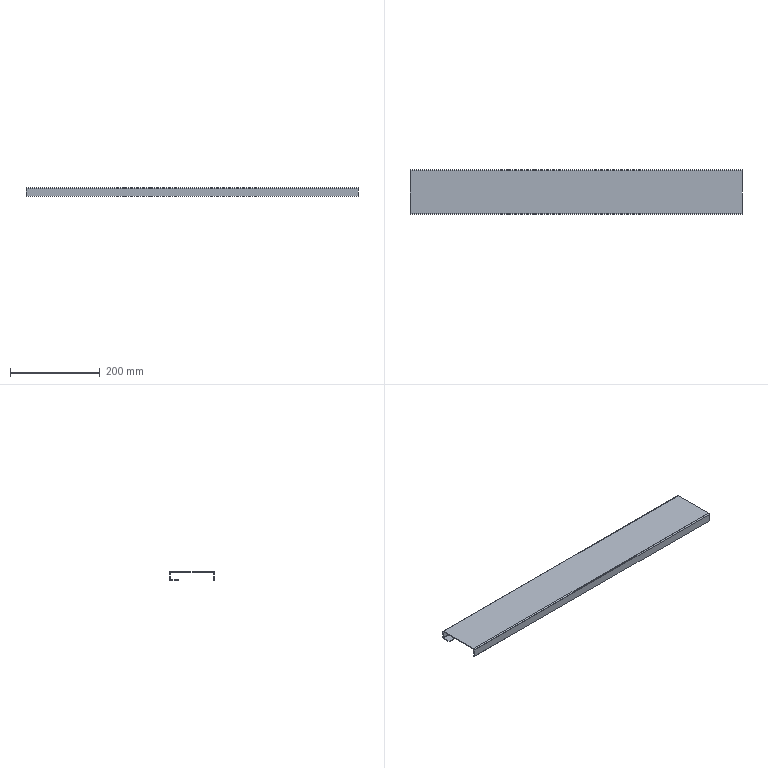Part | STEP file | E3-粉仓护栏10踢脚Plate | 1 solid | 18 faces | box 740.5 x 100 x 20 mm | volume 170219 mm3 | plane 12 | cylinder 6 | commonest cylinder face diameters 2 x3 5 x3
STEP:
#1=CARTESIAN_POINT('',(0.,0.,0.));
#2=DIRECTION('',(0.,0.,1.));
#3=DIRECTION('',(1.,0.,0.));
#4=AXIS2_PLACEMENT_3D('',#1,#2,#3);
#5=CARTESIAN_POINT('',(-370.25,1.5,-2.5));
#6=VERTEX_POINT('',#5);
#7=CARTESIAN_POINT('',(-370.25,1.5,-20.));
#8=VERTEX_POINT('',#7);
#9=CARTESIAN_POINT('',(-370.25,1.5,-2.5));
#10=DIRECTION('',(0.,0.,-1.));
#11=VECTOR('',#10,1.);
#12=LINE('',#9,#11);
#13=CARTESIAN_POINT('',(370.25,1.5,-2.5));
#14=DIRECTION('',(0.,-1.,0.));
#15=DIRECTION('',(0.,0.,1.));
#16=AXIS2_PLACEMENT_3D('',#13,#14,#15);
#17=PLANE('',#16);
#18=CARTESIAN_POINT('',(0.,740.5));
#19=DIRECTION('',(-1.,0.));
#20=VECTOR('',#19,1.);
#21=LINE('',#18,#20);
#22=(GEOMETRIC_REPRESENTATION_CONTEXT(2)PARAMETRIC_REPRESENTATION_CONTEXT()REPRESENTATION_CONTEXT('',''));
#23=DEFINITIONAL_REPRESENTATION('',(#21),#22);
#24=PCURVE('',#17,#23);
#25=CARTESIAN_POINT('',(-370.25,2.5,-2.5));
#26=DIRECTION('',(-1.,0.,0.));
#27=DIRECTION('',(0.,0.,-1.));
#28=AXIS2_PLACEMENT_3D('',#25,#26,#27);
#29=PLANE('',#28);
#30=CARTESIAN_POINT('',(0.,1.));
#31=DIRECTION('',(1.,0.));
#32=VECTOR('',#31,1.);
#33=LINE('',#30,#32);
#34=(GEOMETRIC_REPRESENTATION_CONTEXT(2)PARAMETRIC_REPRESENTATION_CONTEXT()REPRESENTATION_CONTEXT('',''));
#35=DEFINITIONAL_REPRESENTATION('',(#33),#34);
#36=PCURVE('',#29,#35);
#37=SURFACE_CURVE('',#12,(#24,#36),.PCURVE_S1.);
#38=EDGE_CURVE('',#6,#8,#37,.T.);
#39=ORIENTED_EDGE('',*,*,#38,.F.);
#40=CARTESIAN_POINT('',(370.25,1.5,-2.5));
#41=VERTEX_POINT('',#40);
#42=CARTESIAN_POINT('',(370.25,1.5,-2.5));
#43=DIRECTION('',(-1.,0.,0.));
#44=VECTOR('',#43,1.);
#45=LINE('',#42,#44);
#46=CARTESIAN_POINT('',(0.,0.));
#47=DIRECTION('',(0.,1.));
#48=VECTOR('',#47,1.);
#49=LINE('',#46,#48);
#50=(GEOMETRIC_REPRESENTATION_CONTEXT(2)PARAMETRIC_REPRESENTATION_CONTEXT()REPRESENTATION_CONTEXT('',''));
#51=DEFINITIONAL_REPRESENTATION('',(#49),#50);
#52=PCURVE('',#17,#51);
#53=CARTESIAN_POINT('',(370.25,2.5,-2.5));
#54=DIRECTION('',(-1.,0.,0.));
#55=DIRECTION('',(0.,0.,-1.));
#56=AXIS2_PLACEMENT_3D('',#53,#54,#55);
#57=CYLINDRICAL_SURFACE('',#56,1.);
#58=CARTESIAN_POINT('',(1.571,0.));
#59=DIRECTION('',(0.,1.));
#60=VECTOR('',#59,1.);
#61=LINE('',#58,#60);
#62=(GEOMETRIC_REPRESENTATION_CONTEXT(2)PARAMETRIC_REPRESENTATION_CONTEXT()REPRESENTATION_CONTEXT('',''));
#63=DEFINITIONAL_REPRESENTATION('',(#61),#62);
#64=PCURVE('',#57,#63);
#65=SURFACE_CURVE('',#45,(#52,#64),.PCURVE_S1.);
#66=EDGE_CURVE('',#41,#6,#65,.T.);
#67=ORIENTED_EDGE('',*,*,#66,.F.);
#68=CARTESIAN_POINT('',(370.25,1.5,-20.));
#69=VERTEX_POINT('',#68);
#70=CARTESIAN_POINT('',(370.25,1.5,-2.5));
#71=DIRECTION('',(0.,0.,-1.));
#72=VECTOR('',#71,1.);
#73=LINE('',#70,#72);
#74=CARTESIAN_POINT('',(0.,0.));
#75=DIRECTION('',(-1.,0.));
#76=VECTOR('',#75,1.);
#77=LINE('',#74,#76);
#78=(GEOMETRIC_REPRESENTATION_CONTEXT(2)PARAMETRIC_REPRESENTATION_CONTEXT()REPRESENTATION_CONTEXT('',''));
#79=DEFINITIONAL_REPRESENTATION('',(#77),#78);
#80=PCURVE('',#17,#79);
#81=CARTESIAN_POINT('',(370.25,2.5,-2.5));
#82=DIRECTION('',(-1.,0.,0.));
#83=DIRECTION('',(0.,0.,-1.));
#84=AXIS2_PLACEMENT_3D('',#81,#82,#83);
#85=PLANE('',#84);
#86=CARTESIAN_POINT('',(0.,1.));
#87=DIRECTION('',(1.,0.));
#88=VECTOR('',#87,1.);
#89=LINE('',#86,#88);
#90=(GEOMETRIC_REPRESENTATION_CONTEXT(2)PARAMETRIC_REPRESENTATION_CONTEXT()REPRESENTATION_CONTEXT('',''));
#91=DEFINITIONAL_REPRESENTATION('',(#89),#90);
#92=PCURVE('',#85,#91);
#93=SURFACE_CURVE('',#73,(#80,#92),.PCURVE_S1.);
#94=EDGE_CURVE('',#41,#69,#93,.T.);
#95=ORIENTED_EDGE('',*,*,#94,.T.);
#96=CARTESIAN_POINT('',(370.25,1.5,-20.));
#97=DIRECTION('',(-1.,0.,0.));
#98=VECTOR('',#97,1.);
#99=LINE('',#96,#98);
#100=CARTESIAN_POINT('',(-17.5,0.));
#101=DIRECTION('',(0.,1.));
#102=VECTOR('',#101,1.);
#103=LINE('',#100,#102);
#104=(GEOMETRIC_REPRESENTATION_CONTEXT(2)PARAMETRIC_REPRESENTATION_CONTEXT()REPRESENTATION_CONTEXT('',''));
#105=DEFINITIONAL_REPRESENTATION('',(#103),#104);
#106=PCURVE('',#17,#105);
#107=CARTESIAN_POINT('',(370.25,0.,-20.));
#108=DIRECTION('',(0.,0.,-1.));
#109=DIRECTION('',(1.,0.,0.));
#110=AXIS2_PLACEMENT_3D('',#107,#108,#109);
#111=PLANE('',#110);
#112=CARTESIAN_POINT('',(0.,-1.5));
#113=DIRECTION('',(-1.,0.));
#114=VECTOR('',#113,1.);
#115=LINE('',#112,#114);
#116=(GEOMETRIC_REPRESENTATION_CONTEXT(2)PARAMETRIC_REPRESENTATION_CONTEXT()REPRESENTATION_CONTEXT('',''));
#117=DEFINITIONAL_REPRESENTATION('',(#115),#116);
#118=PCURVE('',#111,#117);
#119=SURFACE_CURVE('',#99,(#106,#118),.PCURVE_S1.);
#120=EDGE_CURVE('',#69,#8,#119,.T.);
#121=ORIENTED_EDGE('',*,*,#120,.T.);
#122=EDGE_LOOP('',(#39,#67,#95,#121));
#123=FACE_BOUND('',#122,.T.);
#124=ADVANCED_FACE('',(#123),#17,.F.);
#125=CARTESIAN_POINT('',(-370.25,0.,-20.));
#126=VERTEX_POINT('',#125);
#127=CARTESIAN_POINT('',(-370.25,0.,-20.));
#128=DIRECTION('',(0.,1.,0.));
#129=VECTOR('',#128,1.);
#130=LINE('',#127,#129);
#131=CARTESIAN_POINT('',(-740.5,0.));
#132=DIRECTION('',(0.,-1.));
#133=VECTOR('',#132,1.);
#134=LINE('',#131,#133);
#135=(GEOMETRIC_REPRESENTATION_CONTEXT(2)PARAMETRIC_REPRESENTATION_CONTEXT()REPRESENTATION_CONTEXT('',''));
#136=DEFINITIONAL_REPRESENTATION('',(#134),#135);
#137=PCURVE('',#111,#136);
#138=CARTESIAN_POINT('',(17.5,2.5));
#139=DIRECTION('',(0.,-1.));
#140=VECTOR('',#139,1.);
#141=LINE('',#138,#140);
#142=(GEOMETRIC_REPRESENTATION_CONTEXT(2)PARAMETRIC_REPRESENTATION_CONTEXT()REPRESENTATION_CONTEXT('',''));
#143=DEFINITIONAL_REPRESENTATION('',(#141),#142);
#144=PCURVE('',#29,#143);
#145=SURFACE_CURVE('',#130,(#137,#144),.PCURVE_S1.);
#146=EDGE_CURVE('',#126,#8,#145,.T.);
#147=ORIENTED_EDGE('',*,*,#146,.T.);
#148=ORIENTED_EDGE('',*,*,#120,.F.);
#149=CARTESIAN_POINT('',(370.25,0.,-20.));
#150=VERTEX_POINT('',#149);
#151=CARTESIAN_POINT('',(370.25,0.,-20.));
#152=DIRECTION('',(0.,1.,0.));
#153=VECTOR('',#152,1.);
#154=LINE('',#151,#153);
#155=CARTESIAN_POINT('',(0.,0.));
#156=DIRECTION('',(0.,-1.));
#157=VECTOR('',#156,1.);
#158=LINE('',#155,#157);
#159=(GEOMETRIC_REPRESENTATION_CONTEXT(2)PARAMETRIC_REPRESENTATION_CONTEXT()REPRESENTATION_CONTEXT('',''));
#160=DEFINITIONAL_REPRESENTATION('',(#158),#159);
#161=PCURVE('',#111,#160);
#162=CARTESIAN_POINT('',(17.5,2.5));
#163=DIRECTION('',(0.,-1.));
#164=VECTOR('',#163,1.);
#165=LINE('',#162,#164);
#166=(GEOMETRIC_REPRESENTATION_CONTEXT(2)PARAMETRIC_REPRESENTATION_CONTEXT()REPRESENTATION_CONTEXT('',''));
#167=DEFINITIONAL_REPRESENTATION('',(#165),#166);
#168=PCURVE('',#85,#167);
#169=SURFACE_CURVE('',#154,(#161,#168),.PCURVE_S1.);
#170=EDGE_CURVE('',#150,#69,#169,.T.);
#171=ORIENTED_EDGE('',*,*,#170,.F.);
#172=CARTESIAN_POINT('',(370.25,0.,-20.));
#173=DIRECTION('',(-1.,0.,0.));
#174=VECTOR('',#173,1.);
#175=LINE('',#172,#174);
#176=CARTESIAN_POINT('',(0.,0.));
#177=DIRECTION('',(-1.,0.));
#178=VECTOR('',#177,1.);
#179=LINE('',#176,#178);
#180=(GEOMETRIC_REPRESENTATION_CONTEXT(2)PARAMETRIC_REPRESENTATION_CONTEXT()REPRESENTATION_CONTEXT('',''));
#181=DEFINITIONAL_REPRESENTATION('',(#179),#180);
#182=PCURVE('',#111,#181);
#183=CARTESIAN_POINT('',(370.25,0.,-2.5));
#184=DIRECTION('',(0.,-1.,0.));
#185=DIRECTION('',(0.,0.,1.));
#186=AXIS2_PLACEMENT_3D('',#183,#184,#185);
#187=PLANE('',#186);
#188=CARTESIAN_POINT('',(-17.5,0.));
#189=DIRECTION('',(0.,1.));
#190=VECTOR('',#189,1.);
#191=LINE('',#188,#190);
#192=(GEOMETRIC_REPRESENTATION_CONTEXT(2)PARAMETRIC_REPRESENTATION_CONTEXT()REPRESENTATION_CONTEXT('',''));
#193=DEFINITIONAL_REPRESENTATION('',(#191),#192);
#194=PCURVE('',#187,#193);
#195=SURFACE_CURVE('',#175,(#182,#194),.PCURVE_S1.);
#196=EDGE_CURVE('',#150,#126,#195,.T.);
#197=ORIENTED_EDGE('',*,*,#196,.T.);
#198=EDGE_LOOP('',(#147,#148,#171,#197));
#199=FACE_BOUND('',#198,.T.);
#200=ADVANCED_FACE('',(#199),#111,.T.);
#201=CARTESIAN_POINT('',(-370.25,0.,-2.5));
#202=VERTEX_POINT('',#201);
#203=CARTESIAN_POINT('',(-370.25,0.,-2.5));
#204=DIRECTION('',(0.,0.,-1.));
#205=VECTOR('',#204,1.);
#206=LINE('',#203,#205);
#207=CARTESIAN_POINT('',(0.,740.5));
#208=DIRECTION('',(-1.,0.));
#209=VECTOR('',#208,1.);
#210=LINE('',#207,#209);
#211=(GEOMETRIC_REPRESENTATION_CONTEXT(2)PARAMETRIC_REPRESENTATION_CONTEXT()REPRESENTATION_CONTEXT('',''));
#212=DEFINITIONAL_REPRESENTATION('',(#210),#211);
#213=PCURVE('',#187,#212);
#214=CARTESIAN_POINT('',(0.,2.5));
#215=DIRECTION('',(1.,0.));
#216=VECTOR('',#215,1.);
#217=LINE('',#214,#216);
#218=(GEOMETRIC_REPRESENTATION_CONTEXT(2)PARAMETRIC_REPRESENTATION_CONTEXT()REPRESENTATION_CONTEXT('',''));
#219=DEFINITIONAL_REPRESENTATION('',(#217),#218);
#220=PCURVE('',#29,#219);
#221=SURFACE_CURVE('',#206,(#213,#220),.PCURVE_S1.);
#222=EDGE_CURVE('',#202,#126,#221,.T.);
#223=ORIENTED_EDGE('',*,*,#222,.T.);
#224=ORIENTED_EDGE('',*,*,#196,.F.);
#225=CARTESIAN_POINT('',(370.25,0.,-2.5));
#226=VERTEX_POINT('',#225);
#227=CARTESIAN_POINT('',(370.25,0.,-2.5));
#228=DIRECTION('',(0.,0.,-1.));
#229=VECTOR('',#228,1.);
#230=LINE('',#227,#229);
#231=CARTESIAN_POINT('',(0.,0.));
#232=DIRECTION('',(-1.,0.));
#233=VECTOR('',#232,1.);
#234=LINE('',#231,#233);
#235=(GEOMETRIC_REPRESENTATION_CONTEXT(2)PARAMETRIC_REPRESENTATION_CONTEXT()REPRESENTATION_CONTEXT('',''));
#236=DEFINITIONAL_REPRESENTATION('',(#234),#235);
#237=PCURVE('',#187,#236);
#238=CARTESIAN_POINT('',(0.,2.5));
#239=DIRECTION('',(1.,0.));
#240=VECTOR('',#239,1.);
#241=LINE('',#238,#240);
#242=(GEOMETRIC_REPRESENTATION_CONTEXT(2)PARAMETRIC_REPRESENTATION_CONTEXT()REPRESENTATION_CONTEXT('',''));
#243=DEFINITIONAL_REPRESENTATION('',(#241),#242);
#244=PCURVE('',#85,#243);
#245=SURFACE_CURVE('',#230,(#237,#244),.PCURVE_S1.);
#246=EDGE_CURVE('',#226,#150,#245,.T.);
#247=ORIENTED_EDGE('',*,*,#246,.F.);
#248=CARTESIAN_POINT('',(370.25,0.,-2.5));
#249=DIRECTION('',(-1.,0.,0.));
#250=VECTOR('',#249,1.);
#251=LINE('',#248,#250);
#252=CARTESIAN_POINT('',(0.,0.));
#253=DIRECTION('',(0.,1.));
#254=VECTOR('',#253,1.);
#255=LINE('',#252,#254);
#256=(GEOMETRIC_REPRESENTATION_CONTEXT(2)PARAMETRIC_REPRESENTATION_CONTEXT()REPRESENTATION_CONTEXT('',''));
#257=DEFINITIONAL_REPRESENTATION('',(#255),#256);
#258=PCURVE('',#187,#257);
#259=CARTESIAN_POINT('',(370.25,2.5,-2.5));
#260=DIRECTION('',(-1.,0.,0.));
#261=DIRECTION('',(0.,0.,-1.));
#262=AXIS2_PLACEMENT_3D('',#259,#260,#261);
#263=CYLINDRICAL_SURFACE('',#262,2.5);
#264=CARTESIAN_POINT('',(1.571,0.));
#265=DIRECTION('',(0.,1.));
#266=VECTOR('',#265,1.);
#267=LINE('',#264,#266);
#268=(GEOMETRIC_REPRESENTATION_CONTEXT(2)PARAMETRIC_REPRESENTATION_CONTEXT()REPRESENTATION_CONTEXT('',''));
#269=DEFINITIONAL_REPRESENTATION('',(#267),#268);
#270=PCURVE('',#263,#269);
#271=SURFACE_CURVE('',#251,(#258,#270),.PCURVE_S1.);
#272=EDGE_CURVE('',#226,#202,#271,.T.);
#273=ORIENTED_EDGE('',*,*,#272,.T.);
#274=EDGE_LOOP('',(#223,#224,#247,#273));
#275=FACE_BOUND('',#274,.T.);
#276=ADVANCED_FACE('',(#275),#187,.T.);
#277=CARTESIAN_POINT('',(-370.25,2.5,0.));
#278=VERTEX_POINT('',#277);
#279=CARTESIAN_POINT('',(-370.25,2.5,-2.5));
#280=DIRECTION('',(1.,0.,0.));
#281=DIRECTION('',(0.,0.,-1.));
#282=AXIS2_PLACEMENT_3D('',#279,#280,#281);
#283=CIRCLE('',#282,2.5);
#284=CARTESIAN_POINT('',(6.283,740.5));
#285=DIRECTION('',(-1.,0.));
#286=VECTOR('',#285,1.);
#287=LINE('',#284,#286);
#288=(GEOMETRIC_REPRESENTATION_CONTEXT(2)PARAMETRIC_REPRESENTATION_CONTEXT()REPRESENTATION_CONTEXT('',''));
#289=DEFINITIONAL_REPRESENTATION('',(#287),#288);
#290=PCURVE('',#263,#289);
#291=CARTESIAN_POINT('',(2.5,0.));
#292=CARTESIAN_POINT('',(2.5,-4.33));
#293=CARTESIAN_POINT('',(-1.25,-2.165));
#294=CARTESIAN_POINT('',(-5.,0.));
#295=CARTESIAN_POINT('',(-1.25,2.165));
#296=CARTESIAN_POINT('',(2.5,4.33));
#297=CARTESIAN_POINT('',(2.5,0.));
#298=(BOUNDED_CURVE()B_SPLINE_CURVE(2,(#291,#292,#293,#294,#295,#296,#297),.UNSPECIFIED.,.T.,.F.)B_SPLINE_CURVE_WITH_KNOTS((1,2,2,2,2,1),(-2.094,0.,2.094,4.189,6.283,8.378),.UNSPECIFIED.)CURVE()GEOMETRIC_REPRESENTATION_ITEM()RATIONAL_B_SPLINE_CURVE((1.,0.5,1.,0.5,1.,0.5,1.))REPRESENTATION_ITEM(''));
#299=(GEOMETRIC_REPRESENTATION_CONTEXT(2)PARAMETRIC_REPRESENTATION_CONTEXT()REPRESENTATION_CONTEXT('',''));
#300=DEFINITIONAL_REPRESENTATION('',(#298),#299);
#301=PCURVE('',#29,#300);
#302=SURFACE_CURVE('',#283,(#290,#301),.PCURVE_S1.);
#303=EDGE_CURVE('',#278,#202,#302,.T.);
#304=ORIENTED_EDGE('',*,*,#303,.T.);
#305=ORIENTED_EDGE('',*,*,#272,.F.);
#306=CARTESIAN_POINT('',(370.25,2.5,0.));
#307=VERTEX_POINT('',#306);
#308=CARTESIAN_POINT('',(370.25,2.5,-2.5));
#309=DIRECTION('',(1.,0.,0.));
#310=DIRECTION('',(0.,0.,-1.));
#311=AXIS2_PLACEMENT_3D('',#308,#309,#310);
#312=CIRCLE('',#311,2.5);
#313=CARTESIAN_POINT('',(6.283,0.));
#314=DIRECTION('',(-1.,0.));
#315=VECTOR('',#314,1.);
#316=LINE('',#313,#315);
#317=(GEOMETRIC_REPRESENTATION_CONTEXT(2)PARAMETRIC_REPRESENTATION_CONTEXT()REPRESENTATION_CONTEXT('',''));
#318=DEFINITIONAL_REPRESENTATION('',(#316),#317);
#319=PCURVE('',#263,#318);
#320=CARTESIAN_POINT('',(2.5,0.));
#321=CARTESIAN_POINT('',(2.5,-4.33));
#322=CARTESIAN_POINT('',(-1.25,-2.165));
#323=CARTESIAN_POINT('',(-5.,0.));
#324=CARTESIAN_POINT('',(-1.25,2.165));
#325=CARTESIAN_POINT('',(2.5,4.33));
#326=CARTESIAN_POINT('',(2.5,0.));
#327=(BOUNDED_CURVE()B_SPLINE_CURVE(2,(#320,#321,#322,#323,#324,#325,#326),.UNSPECIFIED.,.T.,.F.)B_SPLINE_CURVE_WITH_KNOTS((1,2,2,2,2,1),(-2.094,0.,2.094,4.189,6.283,8.378),.UNSPECIFIED.)CURVE()GEOMETRIC_REPRESENTATION_ITEM()RATIONAL_B_SPLINE_CURVE((1.,0.5,1.,0.5,1.,0.5,1.))REPRESENTATION_ITEM(''));
#328=(GEOMETRIC_REPRESENTATION_CONTEXT(2)PARAMETRIC_REPRESENTATION_CONTEXT()REPRESENTATION_CONTEXT('',''));
#329=DEFINITIONAL_REPRESENTATION('',(#327),#328);
#330=PCURVE('',#85,#329);
#331=SURFACE_CURVE('',#312,(#319,#330),.PCURVE_S1.);
#332=EDGE_CURVE('',#307,#226,#331,.T.);
#333=ORIENTED_EDGE('',*,*,#332,.F.);
#334=CARTESIAN_POINT('',(370.25,2.5,0.));
#335=DIRECTION('',(-1.,0.,0.));
#336=VECTOR('',#335,1.);
#337=LINE('',#334,#336);
#338=CARTESIAN_POINT('',(3.142,0.));
#339=DIRECTION('',(0.,1.));
#340=VECTOR('',#339,1.);
#341=LINE('',#338,#340);
#342=(GEOMETRIC_REPRESENTATION_CONTEXT(2)PARAMETRIC_REPRESENTATION_CONTEXT()REPRESENTATION_CONTEXT('',''));
#343=DEFINITIONAL_REPRESENTATION('',(#341),#342);
#344=PCURVE('',#263,#343);
#345=CARTESIAN_POINT('',(370.25,2.5,0.));
#346=DIRECTION('',(0.,0.,1.));
#347=DIRECTION('',(-1.,0.,0.));
#348=AXIS2_PLACEMENT_3D('',#345,#346,#347);
#349=PLANE('',#348);
#350=CARTESIAN_POINT('',(0.,0.));
#351=DIRECTION('',(1.,0.));
#352=VECTOR('',#351,1.);
#353=LINE('',#350,#352);
#354=(GEOMETRIC_REPRESENTATION_CONTEXT(2)PARAMETRIC_REPRESENTATION_CONTEXT()REPRESENTATION_CONTEXT('',''));
#355=DEFINITIONAL_REPRESENTATION('',(#353),#354);
#356=PCURVE('',#349,#355);
#357=SURFACE_CURVE('',#337,(#344,#356),.PCURVE_S1.);
#358=EDGE_CURVE('',#307,#278,#357,.T.);
#359=ORIENTED_EDGE('',*,*,#358,.T.);
#360=EDGE_LOOP('',(#304,#305,#333,#359));
#361=FACE_BOUND('',#360,.T.);
#362=ADVANCED_FACE('',(#361),#263,.T.);
#363=CARTESIAN_POINT('',(-370.25,97.5,0.));
#364=VERTEX_POINT('',#363);
#365=CARTESIAN_POINT('',(-370.25,2.5,0.));
#366=DIRECTION('',(0.,-1.,0.));
#367=VECTOR('',#366,1.);
#368=LINE('',#365,#367);
#369=CARTESIAN_POINT('',(740.5,0.));
#370=DIRECTION('',(0.,1.));
#371=VECTOR('',#370,1.);
#372=LINE('',#369,#371);
#373=(GEOMETRIC_REPRESENTATION_CONTEXT(2)PARAMETRIC_REPRESENTATION_CONTEXT()REPRESENTATION_CONTEXT('',''));
#374=DEFINITIONAL_REPRESENTATION('',(#372),#373);
#375=PCURVE('',#349,#374);
#376=CARTESIAN_POINT('',(-2.5,0.));
#377=DIRECTION('',(0.,1.));
#378=VECTOR('',#377,1.);
#379=LINE('',#376,#378);
#380=(GEOMETRIC_REPRESENTATION_CONTEXT(2)PARAMETRIC_REPRESENTATION_CONTEXT()REPRESENTATION_CONTEXT('',''));
#381=DEFINITIONAL_REPRESENTATION('',(#379),#380);
#382=PCURVE('',#29,#381);
#383=SURFACE_CURVE('',#368,(#375,#382),.PCURVE_S1.);
#384=EDGE_CURVE('',#364,#278,#383,.T.);
#385=ORIENTED_EDGE('',*,*,#384,.T.);
#386=ORIENTED_EDGE('',*,*,#358,.F.);
#387=CARTESIAN_POINT('',(370.25,97.5,0.));
#388=VERTEX_POINT('',#387);
#389=CARTESIAN_POINT('',(370.25,2.5,0.));
#390=DIRECTION('',(0.,-1.,0.));
#391=VECTOR('',#390,1.);
#392=LINE('',#389,#391);
#393=CARTESIAN_POINT('',(0.,0.));
#394=DIRECTION('',(0.,1.));
#395=VECTOR('',#394,1.);
#396=LINE('',#393,#395);
#397=(GEOMETRIC_REPRESENTATION_CONTEXT(2)PARAMETRIC_REPRESENTATION_CONTEXT()REPRESENTATION_CONTEXT('',''));
#398=DEFINITIONAL_REPRESENTATION('',(#396),#397);
#399=PCURVE('',#349,#398);
#400=CARTESIAN_POINT('',(-2.5,0.));
#401=DIRECTION('',(0.,1.));
#402=VECTOR('',#401,1.);
#403=LINE('',#400,#402);
#404=(GEOMETRIC_REPRESENTATION_CONTEXT(2)PARAMETRIC_REPRESENTATION_CONTEXT()REPRESENTATION_CONTEXT('',''));
#405=DEFINITIONAL_REPRESENTATION('',(#403),#404);
#406=PCURVE('',#85,#405);
#407=SURFACE_CURVE('',#392,(#399,#406),.PCURVE_S1.);
#408=EDGE_CURVE('',#388,#307,#407,.T.);
#409=ORIENTED_EDGE('',*,*,#408,.F.);
#410=CARTESIAN_POINT('',(370.25,97.5,0.));
#411=DIRECTION('',(-1.,0.,0.));
#412=VECTOR('',#411,1.);
#413=LINE('',#410,#412);
#414=CARTESIAN_POINT('',(0.,-95.));
#415=DIRECTION('',(1.,0.));
#416=VECTOR('',#415,1.);
#417=LINE('',#414,#416);
#418=(GEOMETRIC_REPRESENTATION_CONTEXT(2)PARAMETRIC_REPRESENTATION_CONTEXT()REPRESENTATION_CONTEXT('',''));
#419=DEFINITIONAL_REPRESENTATION('',(#417),#418);
#420=PCURVE('',#349,#419);
#421=CARTESIAN_POINT('',(370.25,97.5,-2.5));
#422=DIRECTION('',(-1.,0.,0.));
#423=DIRECTION('',(0.,0.,-1.));
#424=AXIS2_PLACEMENT_3D('',#421,#422,#423);
#425=CYLINDRICAL_SURFACE('',#424,2.5);
#426=CARTESIAN_POINT('',(3.142,0.));
#427=DIRECTION('',(0.,1.));
#428=VECTOR('',#427,1.);
#429=LINE('',#426,#428);
#430=(GEOMETRIC_REPRESENTATION_CONTEXT(2)PARAMETRIC_REPRESENTATION_CONTEXT()REPRESENTATION_CONTEXT('',''));
#431=DEFINITIONAL_REPRESENTATION('',(#429),#430);
#432=PCURVE('',#425,#431);
#433=SURFACE_CURVE('',#413,(#420,#432),.PCURVE_S1.);
#434=EDGE_CURVE('',#388,#364,#433,.T.);
#435=ORIENTED_EDGE('',*,*,#434,.T.);
#436=EDGE_LOOP('',(#385,#386,#409,#435));
#437=FACE_BOUND('',#436,.T.);
#438=ADVANCED_FACE('',(#437),#349,.T.);
#439=CARTESIAN_POINT('',(-370.25,100.,-2.5));
#440=VERTEX_POINT('',#439);
#441=CARTESIAN_POINT('',(-370.25,97.5,-2.5));
#442=DIRECTION('',(1.,0.,0.));
#443=DIRECTION('',(0.,0.,1.));
#444=AXIS2_PLACEMENT_3D('',#441,#442,#443);
#445=CIRCLE('',#444,2.5);
#446=CARTESIAN_POINT('',(9.425,740.5));
#447=DIRECTION('',(-1.,0.));
#448=VECTOR('',#447,1.);
#449=LINE('',#446,#448);
#450=(GEOMETRIC_REPRESENTATION_CONTEXT(2)PARAMETRIC_REPRESENTATION_CONTEXT()REPRESENTATION_CONTEXT('',''));
#451=DEFINITIONAL_REPRESENTATION('',(#449),#450);
#452=PCURVE('',#425,#451);
#453=CARTESIAN_POINT('',(-2.5,-95.));
#454=CARTESIAN_POINT('',(-2.5,-90.67));
#455=CARTESIAN_POINT('',(1.25,-92.835));
#456=CARTESIAN_POINT('',(5.,-95.));
#457=CARTESIAN_POINT('',(1.25,-97.165));
#458=CARTESIAN_POINT('',(-2.5,-99.33));
#459=CARTESIAN_POINT('',(-2.5,-95.));
#460=(BOUNDED_CURVE()B_SPLINE_CURVE(2,(#453,#454,#455,#456,#457,#458,#459),.UNSPECIFIED.,.T.,.F.)B_SPLINE_CURVE_WITH_KNOTS((1,2,2,2,2,1),(-2.094,0.,2.094,4.189,6.283,8.378),.UNSPECIFIED.)CURVE()GEOMETRIC_REPRESENTATION_ITEM()RATIONAL_B_SPLINE_CURVE((1.,0.5,1.,0.5,1.,0.5,1.))REPRESENTATION_ITEM(''));
#461=(GEOMETRIC_REPRESENTATION_CONTEXT(2)PARAMETRIC_REPRESENTATION_CONTEXT()REPRESENTATION_CONTEXT('',''));
#462=DEFINITIONAL_REPRESENTATION('',(#460),#461);
#463=PCURVE('',#29,#462);
#464=SURFACE_CURVE('',#445,(#452,#463),.PCURVE_S1.);
#465=EDGE_CURVE('',#440,#364,#464,.T.);
#466=ORIENTED_EDGE('',*,*,#465,.T.);
#467=ORIENTED_EDGE('',*,*,#434,.F.);
#468=CARTESIAN_POINT('',(370.25,100.,-2.5));
#469=VERTEX_POINT('',#468);
#470=CARTESIAN_POINT('',(370.25,97.5,-2.5));
#471=DIRECTION('',(1.,0.,0.));
#472=DIRECTION('',(0.,0.,1.));
#473=AXIS2_PLACEMENT_3D('',#470,#471,#472);
#474=CIRCLE('',#473,2.5);
#475=CARTESIAN_POINT('',(9.425,0.));
#476=DIRECTION('',(-1.,0.));
#477=VECTOR('',#476,1.);
#478=LINE('',#475,#477);
#479=(GEOMETRIC_REPRESENTATION_CONTEXT(2)PARAMETRIC_REPRESENTATION_CONTEXT()REPRESENTATION_CONTEXT('',''));
#480=DEFINITIONAL_REPRESENTATION('',(#478),#479);
#481=PCURVE('',#425,#480);
#482=CARTESIAN_POINT('',(-2.5,-95.));
#483=CARTESIAN_POINT('',(-2.5,-90.67));
#484=CARTESIAN_POINT('',(1.25,-92.835));
#485=CARTESIAN_POINT('',(5.,-95.));
#486=CARTESIAN_POINT('',(1.25,-97.165));
#487=CARTESIAN_POINT('',(-2.5,-99.33));
#488=CARTESIAN_POINT('',(-2.5,-95.));
#489=(BOUNDED_CURVE()B_SPLINE_CURVE(2,(#482,#483,#484,#485,#486,#487,#488),.UNSPECIFIED.,.T.,.F.)B_SPLINE_CURVE_WITH_KNOTS((1,2,2,2,2,1),(-2.094,0.,2.094,4.189,6.283,8.378),.UNSPECIFIED.)CURVE()GEOMETRIC_REPRESENTATION_ITEM()RATIONAL_B_SPLINE_CURVE((1.,0.5,1.,0.5,1.,0.5,1.))REPRESENTATION_ITEM(''));
#490=(GEOMETRIC_REPRESENTATION_CONTEXT(2)PARAMETRIC_REPRESENTATION_CONTEXT()REPRESENTATION_CONTEXT('',''));
#491=DEFINITIONAL_REPRESENTATION('',(#489),#490);
#492=PCURVE('',#85,#491);
#493=SURFACE_CURVE('',#474,(#481,#492),.PCURVE_S1.);
#494=EDGE_CURVE('',#469,#388,#493,.T.);
#495=ORIENTED_EDGE('',*,*,#494,.F.);
#496=CARTESIAN_POINT('',(370.25,100.,-2.5));
#497=DIRECTION('',(-1.,0.,0.));
#498=VECTOR('',#497,1.);
#499=LINE('',#496,#498);
#500=CARTESIAN_POINT('',(4.712,0.));
#501=DIRECTION('',(0.,1.));
#502=VECTOR('',#501,1.);
#503=LINE('',#500,#502);
#504=(GEOMETRIC_REPRESENTATION_CONTEXT(2)PARAMETRIC_REPRESENTATION_CONTEXT()REPRESENTATION_CONTEXT('',''));
#505=DEFINITIONAL_REPRESENTATION('',(#503),#504);
#506=PCURVE('',#425,#505);
#507=CARTESIAN_POINT('',(370.25,100.,-2.5));
#508=DIRECTION('',(0.,1.,0.));
#509=DIRECTION('',(0.,0.,-1.));
#510=AXIS2_PLACEMENT_3D('',#507,#508,#509);
#511=PLANE('',#510);
#512=CARTESIAN_POINT('',(0.,0.));
#513=DIRECTION('',(0.,1.));
#514=VECTOR('',#513,1.);
#515=LINE('',#512,#514);
#516=(GEOMETRIC_REPRESENTATION_CONTEXT(2)PARAMETRIC_REPRESENTATION_CONTEXT()REPRESENTATION_CONTEXT('',''));
#517=DEFINITIONAL_REPRESENTATION('',(#515),#516);
#518=PCURVE('',#511,#517);
#519=SURFACE_CURVE('',#499,(#506,#518),.PCURVE_S1.);
#520=EDGE_CURVE('',#469,#440,#519,.T.);
#521=ORIENTED_EDGE('',*,*,#520,.T.);
#522=EDGE_LOOP('',(#466,#467,#495,#521));
#523=FACE_BOUND('',#522,.T.);
#524=ADVANCED_FACE('',(#523),#425,.T.);
#525=CARTESIAN_POINT('',(-370.25,100.,-17.5));
#526=VERTEX_POINT('',#525);
#527=CARTESIAN_POINT('',(-370.25,100.,-2.5));
#528=DIRECTION('',(0.,0.,1.));
#529=VECTOR('',#528,1.);
#530=LINE('',#527,#529);
#531=CARTESIAN_POINT('',(0.,740.5));
#532=DIRECTION('',(-1.,0.));
#533=VECTOR('',#532,1.);
#534=LINE('',#531,#533);
#535=(GEOMETRIC_REPRESENTATION_CONTEXT(2)PARAMETRIC_REPRESENTATION_CONTEXT()REPRESENTATION_CONTEXT('',''));
#536=DEFINITIONAL_REPRESENTATION('',(#534),#535);
#537=PCURVE('',#511,#536);
#538=CARTESIAN_POINT('',(0.,-97.5));
#539=DIRECTION('',(-1.,0.));
#540=VECTOR('',#539,1.);
#541=LINE('',#538,#540);
#542=(GEOMETRIC_REPRESENTATION_CONTEXT(2)PARAMETRIC_REPRESENTATION_CONTEXT()REPRESENTATION_CONTEXT('',''));
#543=DEFINITIONAL_REPRESENTATION('',(#541),#542);
#544=PCURVE('',#29,#543);
#545=SURFACE_CURVE('',#530,(#537,#544),.PCURVE_S1.);
#546=EDGE_CURVE('',#526,#440,#545,.T.);
#547=ORIENTED_EDGE('',*,*,#546,.T.);
#548=ORIENTED_EDGE('',*,*,#520,.F.);
#549=CARTESIAN_POINT('',(370.25,100.,-17.5));
#550=VERTEX_POINT('',#549);
#551=CARTESIAN_POINT('',(370.25,100.,-2.5));
#552=DIRECTION('',(0.,0.,1.));
#553=VECTOR('',#552,1.);
#554=LINE('',#551,#553);
#555=CARTESIAN_POINT('',(0.,0.));
#556=DIRECTION('',(-1.,0.));
#557=VECTOR('',#556,1.);
#558=LINE('',#555,#557);
#559=(GEOMETRIC_REPRESENTATION_CONTEXT(2)PARAMETRIC_REPRESENTATION_CONTEXT()REPRESENTATION_CONTEXT('',''));
#560=DEFINITIONAL_REPRESENTATION('',(#558),#559);
#561=PCURVE('',#511,#560);
#562=CARTESIAN_POINT('',(0.,-97.5));
#563=DIRECTION('',(-1.,0.));
#564=VECTOR('',#563,1.);
#565=LINE('',#562,#564);
#566=(GEOMETRIC_REPRESENTATION_CONTEXT(2)PARAMETRIC_REPRESENTATION_CONTEXT()REPRESENTATION_CONTEXT('',''));
#567=DEFINITIONAL_REPRESENTATION('',(#565),#566);
#568=PCURVE('',#85,#567);
#569=SURFACE_CURVE('',#554,(#561,#568),.PCURVE_S1.);
#570=EDGE_CURVE('',#550,#469,#569,.T.);
#571=ORIENTED_EDGE('',*,*,#570,.F.);
#572=CARTESIAN_POINT('',(370.25,100.,-17.5));
#573=DIRECTION('',(-1.,0.,0.));
#574=VECTOR('',#573,1.);
#575=LINE('',#572,#574);
#576=CARTESIAN_POINT('',(15.,0.));
#577=DIRECTION('',(0.,1.));
#578=VECTOR('',#577,1.);
#579=LINE('',#576,#578);
#580=(GEOMETRIC_REPRESENTATION_CONTEXT(2)PARAMETRIC_REPRESENTATION_CONTEXT()REPRESENTATION_CONTEXT('',''));
#581=DEFINITIONAL_REPRESENTATION('',(#579),#580);
#582=PCURVE('',#511,#581);
#583=CARTESIAN_POINT('',(370.25,97.5,-17.5));
#584=DIRECTION('',(-1.,0.,0.));
#585=DIRECTION('',(0.,0.,-1.));
#586=AXIS2_PLACEMENT_3D('',#583,#584,#585);
#587=CYLINDRICAL_SURFACE('',#586,2.5);
#588=CARTESIAN_POINT('',(4.712,0.));
#589=DIRECTION('',(0.,1.));
#590=VECTOR('',#589,1.);
#591=LINE('',#588,#590);
#592=(GEOMETRIC_REPRESENTATION_CONTEXT(2)PARAMETRIC_REPRESENTATION_CONTEXT()REPRESENTATION_CONTEXT('',''));
#593=DEFINITIONAL_REPRESENTATION('',(#591),#592);
#594=PCURVE('',#587,#593);
#595=SURFACE_CURVE('',#575,(#582,#594),.PCURVE_S1.);
#596=EDGE_CURVE('',#550,#526,#595,.T.);
#597=ORIENTED_EDGE('',*,*,#596,.T.);
#598=EDGE_LOOP('',(#547,#548,#571,#597));
#599=FACE_BOUND('',#598,.T.);
#600=ADVANCED_FACE('',(#599),#511,.T.);
#601=CARTESIAN_POINT('',(-370.25,97.5,-20.));
#602=VERTEX_POINT('',#601);
#603=CARTESIAN_POINT('',(-370.25,97.5,-17.5));
#604=DIRECTION('',(1.,0.,0.));
#605=DIRECTION('',(0.,0.,1.));
#606=AXIS2_PLACEMENT_3D('',#603,#604,#605);
#607=CIRCLE('',#606,2.5);
#608=CARTESIAN_POINT('',(9.425,740.5));
#609=DIRECTION('',(-1.,0.));
#610=VECTOR('',#609,1.);
#611=LINE('',#608,#610);
#612=(GEOMETRIC_REPRESENTATION_CONTEXT(2)PARAMETRIC_REPRESENTATION_CONTEXT()REPRESENTATION_CONTEXT('',''));
#613=DEFINITIONAL_REPRESENTATION('',(#611),#612);
#614=PCURVE('',#587,#613);
#615=CARTESIAN_POINT('',(12.5,-95.));
#616=CARTESIAN_POINT('',(12.5,-90.67));
#617=CARTESIAN_POINT('',(16.25,-92.835));
#618=CARTESIAN_POINT('',(20.,-95.));
#619=CARTESIAN_POINT('',(16.25,-97.165));
#620=CARTESIAN_POINT('',(12.5,-99.33));
#621=CARTESIAN_POINT('',(12.5,-95.));
#622=(BOUNDED_CURVE()B_SPLINE_CURVE(2,(#615,#616,#617,#618,#619,#620,#621),.UNSPECIFIED.,.T.,.F.)B_SPLINE_CURVE_WITH_KNOTS((1,2,2,2,2,1),(-2.094,0.,2.094,4.189,6.283,8.378),.UNSPECIFIED.)CURVE()GEOMETRIC_REPRESENTATION_ITEM()RATIONAL_B_SPLINE_CURVE((1.,0.5,1.,0.5,1.,0.5,1.))REPRESENTATION_ITEM(''));
#623=(GEOMETRIC_REPRESENTATION_CONTEXT(2)PARAMETRIC_REPRESENTATION_CONTEXT()REPRESENTATION_CONTEXT('',''));
#624=DEFINITIONAL_REPRESENTATION('',(#622),#623);
#625=PCURVE('',#29,#624);
#626=SURFACE_CURVE('',#607,(#614,#625),.PCURVE_S1.);
#627=EDGE_CURVE('',#602,#526,#626,.T.);
#628=ORIENTED_EDGE('',*,*,#627,.T.);
#629=ORIENTED_EDGE('',*,*,#596,.F.);
#630=CARTESIAN_POINT('',(370.25,97.5,-20.));
#631=VERTEX_POINT('',#630);
#632=CARTESIAN_POINT('',(370.25,97.5,-17.5));
#633=DIRECTION('',(1.,0.,0.));
#634=DIRECTION('',(0.,0.,1.));
#635=AXIS2_PLACEMENT_3D('',#632,#633,#634);
#636=CIRCLE('',#635,2.5);
#637=CARTESIAN_POINT('',(9.425,0.));
#638=DIRECTION('',(-1.,0.));
#639=VECTOR('',#638,1.);
#640=LINE('',#637,#639);
#641=(GEOMETRIC_REPRESENTATION_CONTEXT(2)PARAMETRIC_REPRESENTATION_CONTEXT()REPRESENTATION_CONTEXT('',''));
#642=DEFINITIONAL_REPRESENTATION('',(#640),#641);
#643=PCURVE('',#587,#642);
#644=CARTESIAN_POINT('',(12.5,-95.));
#645=CARTESIAN_POINT('',(12.5,-90.67));
#646=CARTESIAN_POINT('',(16.25,-92.835));
#647=CARTESIAN_POINT('',(20.,-95.));
#648=CARTESIAN_POINT('',(16.25,-97.165));
#649=CARTESIAN_POINT('',(12.5,-99.33));
#650=CARTESIAN_POINT('',(12.5,-95.));
#651=(BOUNDED_CURVE()B_SPLINE_CURVE(2,(#644,#645,#646,#647,#648,#649,#650),.UNSPECIFIED.,.T.,.F.)B_SPLINE_CURVE_WITH_KNOTS((1,2,2,2,2,1),(-2.094,0.,2.094,4.189,6.283,8.378),.UNSPECIFIED.)CURVE()GEOMETRIC_REPRESENTATION_ITEM()RATIONAL_B_SPLINE_CURVE((1.,0.5,1.,0.5,1.,0.5,1.))REPRESENTATION_ITEM(''));
#652=(GEOMETRIC_REPRESENTATION_CONTEXT(2)PARAMETRIC_REPRESENTATION_CONTEXT()REPRESENTATION_CONTEXT('',''));
#653=DEFINITIONAL_REPRESENTATION('',(#651),#652);
#654=PCURVE('',#85,#653);
#655=SURFACE_CURVE('',#636,(#643,#654),.PCURVE_S1.);
#656=EDGE_CURVE('',#631,#550,#655,.T.);
#657=ORIENTED_EDGE('',*,*,#656,.F.);
#658=CARTESIAN_POINT('',(370.25,97.5,-20.));
#659=DIRECTION('',(-1.,0.,0.));
#660=VECTOR('',#659,1.);
#661=LINE('',#658,#660);
#662=CARTESIAN_POINT('',(6.283,0.));
#663=DIRECTION('',(0.,1.));
#664=VECTOR('',#663,1.);
#665=LINE('',#662,#664);
#666=(GEOMETRIC_REPRESENTATION_CONTEXT(2)PARAMETRIC_REPRESENTATION_CONTEXT()REPRESENTATION_CONTEXT('',''));
#667=DEFINITIONAL_REPRESENTATION('',(#665),#666);
#668=PCURVE('',#587,#667);
#669=CARTESIAN_POINT('',(370.25,97.5,-20.));
#670=DIRECTION('',(0.,0.,-1.));
#671=DIRECTION('',(1.,0.,0.));
#672=AXIS2_PLACEMENT_3D('',#669,#670,#671);
#673=PLANE('',#672);
#674=CARTESIAN_POINT('',(0.,0.));
#675=DIRECTION('',(-1.,0.));
#676=VECTOR('',#675,1.);
#677=LINE('',#674,#676);
#678=(GEOMETRIC_REPRESENTATION_CONTEXT(2)PARAMETRIC_REPRESENTATION_CONTEXT()REPRESENTATION_CONTEXT('',''));
#679=DEFINITIONAL_REPRESENTATION('',(#677),#678);
#680=PCURVE('',#673,#679);
#681=SURFACE_CURVE('',#661,(#668,#680),.PCURVE_S1.);
#682=EDGE_CURVE('',#631,#602,#681,.T.);
#683=ORIENTED_EDGE('',*,*,#682,.T.);
#684=EDGE_LOOP('',(#628,#629,#657,#683));
#685=FACE_BOUND('',#684,.T.);
#686=ADVANCED_FACE('',(#685),#587,.T.);
#687=CARTESIAN_POINT('',(-370.25,80.,-20.));
#688=VERTEX_POINT('',#687);
#689=CARTESIAN_POINT('',(-370.25,97.5,-20.));
#690=DIRECTION('',(0.,1.,0.));
#691=VECTOR('',#690,1.);
#692=LINE('',#689,#691);
#693=CARTESIAN_POINT('',(-740.5,0.));
#694=DIRECTION('',(0.,-1.));
#695=VECTOR('',#694,1.);
#696=LINE('',#693,#695);
#697=(GEOMETRIC_REPRESENTATION_CONTEXT(2)PARAMETRIC_REPRESENTATION_CONTEXT()REPRESENTATION_CONTEXT('',''));
#698=DEFINITIONAL_REPRESENTATION('',(#696),#697);
#699=PCURVE('',#673,#698);
#700=CARTESIAN_POINT('',(17.5,-95.));
#701=DIRECTION('',(0.,-1.));
#702=VECTOR('',#701,1.);
#703=LINE('',#700,#702);
#704=(GEOMETRIC_REPRESENTATION_CONTEXT(2)PARAMETRIC_REPRESENTATION_CONTEXT()REPRESENTATION_CONTEXT('',''));
#705=DEFINITIONAL_REPRESENTATION('',(#703),#704);
#706=PCURVE('',#29,#705);
#707=SURFACE_CURVE('',#692,(#699,#706),.PCURVE_S1.);
#708=EDGE_CURVE('',#688,#602,#707,.T.);
#709=ORIENTED_EDGE('',*,*,#708,.T.);
#710=ORIENTED_EDGE('',*,*,#682,.F.);
#711=CARTESIAN_POINT('',(370.25,80.,-20.));
#712=VERTEX_POINT('',#711);
#713=CARTESIAN_POINT('',(370.25,97.5,-20.));
#714=DIRECTION('',(0.,1.,0.));
#715=VECTOR('',#714,1.);
#716=LINE('',#713,#715);
#717=CARTESIAN_POINT('',(0.,0.));
#718=DIRECTION('',(0.,-1.));
#719=VECTOR('',#718,1.);
#720=LINE('',#717,#719);
#721=(GEOMETRIC_REPRESENTATION_CONTEXT(2)PARAMETRIC_REPRESENTATION_CONTEXT()REPRESENTATION_CONTEXT('',''));
#722=DEFINITIONAL_REPRESENTATION('',(#720),#721);
#723=PCURVE('',#673,#722);
#724=CARTESIAN_POINT('',(17.5,-95.));
#725=DIRECTION('',(0.,-1.));
#726=VECTOR('',#725,1.);
#727=LINE('',#724,#726);
#728=(GEOMETRIC_REPRESENTATION_CONTEXT(2)PARAMETRIC_REPRESENTATION_CONTEXT()REPRESENTATION_CONTEXT('',''));
#729=DEFINITIONAL_REPRESENTATION('',(#727),#728);
#730=PCURVE('',#85,#729);
#731=SURFACE_CURVE('',#716,(#723,#730),.PCURVE_S1.);
#732=EDGE_CURVE('',#712,#631,#731,.T.);
#733=ORIENTED_EDGE('',*,*,#732,.F.);
#734=CARTESIAN_POINT('',(370.25,80.,-20.));
#735=DIRECTION('',(-1.,0.,0.));
#736=VECTOR('',#735,1.);
#737=LINE('',#734,#736);
#738=CARTESIAN_POINT('',(0.,17.5));
#739=DIRECTION('',(-1.,0.));
#740=VECTOR('',#739,1.);
#741=LINE('',#738,#740);
#742=(GEOMETRIC_REPRESENTATION_CONTEXT(2)PARAMETRIC_REPRESENTATION_CONTEXT()REPRESENTATION_CONTEXT('',''));
#743=DEFINITIONAL_REPRESENTATION('',(#741),#742);
#744=PCURVE('',#673,#743);
#745=CARTESIAN_POINT('',(370.25,80.,-18.5));
#746=DIRECTION('',(0.,-1.,0.));
#747=DIRECTION('',(0.,0.,1.));
#748=AXIS2_PLACEMENT_3D('',#745,#746,#747);
#749=PLANE('',#748);
#750=CARTESIAN_POINT('',(-1.5,0.));
#751=DIRECTION('',(0.,1.));
#752=VECTOR('',#751,1.);
#753=LINE('',#750,#752);
#754=(GEOMETRIC_REPRESENTATION_CONTEXT(2)PARAMETRIC_REPRESENTATION_CONTEXT()REPRESENTATION_CONTEXT('',''));
#755=DEFINITIONAL_REPRESENTATION('',(#753),#754);
#756=PCURVE('',#749,#755);
#757=SURFACE_CURVE('',#737,(#744,#756),.PCURVE_S1.);
#758=EDGE_CURVE('',#712,#688,#757,.T.);
#759=ORIENTED_EDGE('',*,*,#758,.T.);
#760=EDGE_LOOP('',(#709,#710,#733,#759));
#761=FACE_BOUND('',#760,.T.);
#762=ADVANCED_FACE('',(#761),#673,.T.);
#763=CARTESIAN_POINT('',(-370.25,80.,-18.5));
#764=VERTEX_POINT('',#763);
#765=CARTESIAN_POINT('',(-370.25,80.,-18.5));
#766=DIRECTION('',(0.,0.,-1.));
#767=VECTOR('',#766,1.);
#768=LINE('',#765,#767);
#769=CARTESIAN_POINT('',(0.,740.5));
#770=DIRECTION('',(-1.,0.));
#771=VECTOR('',#770,1.);
#772=LINE('',#769,#771);
#773=(GEOMETRIC_REPRESENTATION_CONTEXT(2)PARAMETRIC_REPRESENTATION_CONTEXT()REPRESENTATION_CONTEXT('',''));
#774=DEFINITIONAL_REPRESENTATION('',(#772),#773);
#775=PCURVE('',#749,#774);
#776=CARTESIAN_POINT('',(16.,-77.5));
#777=DIRECTION('',(1.,0.));
#778=VECTOR('',#777,1.);
#779=LINE('',#776,#778);
#780=(GEOMETRIC_REPRESENTATION_CONTEXT(2)PARAMETRIC_REPRESENTATION_CONTEXT()REPRESENTATION_CONTEXT('',''));
#781=DEFINITIONAL_REPRESENTATION('',(#779),#780);
#782=PCURVE('',#29,#781);
#783=SURFACE_CURVE('',#768,(#775,#782),.PCURVE_S1.);
#784=EDGE_CURVE('',#764,#688,#783,.T.);
#785=ORIENTED_EDGE('',*,*,#784,.T.);
#786=ORIENTED_EDGE('',*,*,#758,.F.);
#787=CARTESIAN_POINT('',(370.25,80.,-18.5));
#788=VERTEX_POINT('',#787);
#789=CARTESIAN_POINT('',(370.25,80.,-18.5));
#790=DIRECTION('',(0.,0.,-1.));
#791=VECTOR('',#790,1.);
#792=LINE('',#789,#791);
#793=CARTESIAN_POINT('',(0.,0.));
#794=DIRECTION('',(-1.,0.));
#795=VECTOR('',#794,1.);
#796=LINE('',#793,#795);
#797=(GEOMETRIC_REPRESENTATION_CONTEXT(2)PARAMETRIC_REPRESENTATION_CONTEXT()REPRESENTATION_CONTEXT('',''));
#798=DEFINITIONAL_REPRESENTATION('',(#796),#797);
#799=PCURVE('',#749,#798);
#800=CARTESIAN_POINT('',(16.,-77.5));
#801=DIRECTION('',(1.,0.));
#802=VECTOR('',#801,1.);
#803=LINE('',#800,#802);
#804=(GEOMETRIC_REPRESENTATION_CONTEXT(2)PARAMETRIC_REPRESENTATION_CONTEXT()REPRESENTATION_CONTEXT('',''));
#805=DEFINITIONAL_REPRESENTATION('',(#803),#804);
#806=PCURVE('',#85,#805);
#807=SURFACE_CURVE('',#792,(#799,#806),.PCURVE_S1.);
#808=EDGE_CURVE('',#788,#712,#807,.T.);
#809=ORIENTED_EDGE('',*,*,#808,.F.);
#810=CARTESIAN_POINT('',(370.25,80.,-18.5));
#811=DIRECTION('',(-1.,0.,0.));
#812=VECTOR('',#811,1.);
#813=LINE('',#810,#812);
#814=CARTESIAN_POINT('',(0.,0.));
#815=DIRECTION('',(0.,1.));
#816=VECTOR('',#815,1.);
#817=LINE('',#814,#816);
#818=(GEOMETRIC_REPRESENTATION_CONTEXT(2)PARAMETRIC_REPRESENTATION_CONTEXT()REPRESENTATION_CONTEXT('',''));
#819=DEFINITIONAL_REPRESENTATION('',(#817),#818);
#820=PCURVE('',#749,#819);
#821=CARTESIAN_POINT('',(370.25,97.5,-18.5));
#822=DIRECTION('',(0.,0.,-1.));
#823=DIRECTION('',(1.,0.,0.));
#824=AXIS2_PLACEMENT_3D('',#821,#822,#823);
#825=PLANE('',#824);
#826=CARTESIAN_POINT('',(0.,17.5));
#827=DIRECTION('',(-1.,0.));
#828=VECTOR('',#827,1.);
#829=LINE('',#826,#828);
#830=(GEOMETRIC_REPRESENTATION_CONTEXT(2)PARAMETRIC_REPRESENTATION_CONTEXT()REPRESENTATION_CONTEXT('',''));
#831=DEFINITIONAL_REPRESENTATION('',(#829),#830);
#832=PCURVE('',#825,#831);
#833=SURFACE_CURVE('',#813,(#820,#832),.PCURVE_S1.);
#834=EDGE_CURVE('',#788,#764,#833,.T.);
#835=ORIENTED_EDGE('',*,*,#834,.T.);
#836=EDGE_LOOP('',(#785,#786,#809,#835));
#837=FACE_BOUND('',#836,.T.);
#838=ADVANCED_FACE('',(#837),#749,.T.);
#839=CARTESIAN_POINT('',(-370.25,97.5,-18.5));
#840=VERTEX_POINT('',#839);
#841=CARTESIAN_POINT('',(-370.25,97.5,-18.5));
#842=DIRECTION('',(0.,1.,0.));
#843=VECTOR('',#842,1.);
#844=LINE('',#841,#843);
#845=CARTESIAN_POINT('',(-740.5,0.));
#846=DIRECTION('',(0.,-1.));
#847=VECTOR('',#846,1.);
#848=LINE('',#845,#847);
#849=(GEOMETRIC_REPRESENTATION_CONTEXT(2)PARAMETRIC_REPRESENTATION_CONTEXT()REPRESENTATION_CONTEXT('',''));
#850=DEFINITIONAL_REPRESENTATION('',(#848),#849);
#851=PCURVE('',#825,#850);
#852=CARTESIAN_POINT('',(16.,-95.));
#853=DIRECTION('',(0.,-1.));
#854=VECTOR('',#853,1.);
#855=LINE('',#852,#854);
#856=(GEOMETRIC_REPRESENTATION_CONTEXT(2)PARAMETRIC_REPRESENTATION_CONTEXT()REPRESENTATION_CONTEXT('',''));
#857=DEFINITIONAL_REPRESENTATION('',(#855),#856);
#858=PCURVE('',#29,#857);
#859=SURFACE_CURVE('',#844,(#851,#858),.PCURVE_S1.);
#860=EDGE_CURVE('',#764,#840,#859,.T.);
#861=ORIENTED_EDGE('',*,*,#860,.F.);
#862=ORIENTED_EDGE('',*,*,#834,.F.);
#863=CARTESIAN_POINT('',(370.25,97.5,-18.5));
#864=VERTEX_POINT('',#863);
#865=CARTESIAN_POINT('',(370.25,97.5,-18.5));
#866=DIRECTION('',(0.,1.,0.));
#867=VECTOR('',#866,1.);
#868=LINE('',#865,#867);
#869=CARTESIAN_POINT('',(0.,0.));
#870=DIRECTION('',(0.,-1.));
#871=VECTOR('',#870,1.);
#872=LINE('',#869,#871);
#873=(GEOMETRIC_REPRESENTATION_CONTEXT(2)PARAMETRIC_REPRESENTATION_CONTEXT()REPRESENTATION_CONTEXT('',''));
#874=DEFINITIONAL_REPRESENTATION('',(#872),#873);
#875=PCURVE('',#825,#874);
#876=CARTESIAN_POINT('',(16.,-95.));
#877=DIRECTION('',(0.,-1.));
#878=VECTOR('',#877,1.);
#879=LINE('',#876,#878);
#880=(GEOMETRIC_REPRESENTATION_CONTEXT(2)PARAMETRIC_REPRESENTATION_CONTEXT()REPRESENTATION_CONTEXT('',''));
#881=DEFINITIONAL_REPRESENTATION('',(#879),#880);
#882=PCURVE('',#85,#881);
#883=SURFACE_CURVE('',#868,(#875,#882),.PCURVE_S1.);
#884=EDGE_CURVE('',#788,#864,#883,.T.);
#885=ORIENTED_EDGE('',*,*,#884,.T.);
#886=CARTESIAN_POINT('',(370.25,97.5,-18.5));
#887=DIRECTION('',(-1.,0.,0.));
#888=VECTOR('',#887,1.);
#889=LINE('',#886,#888);
#890=CARTESIAN_POINT('',(0.,0.));
#891=DIRECTION('',(-1.,0.));
#892=VECTOR('',#891,1.);
#893=LINE('',#890,#892);
#894=(GEOMETRIC_REPRESENTATION_CONTEXT(2)PARAMETRIC_REPRESENTATION_CONTEXT()REPRESENTATION_CONTEXT('',''));
#895=DEFINITIONAL_REPRESENTATION('',(#893),#894);
#896=PCURVE('',#825,#895);
#897=CARTESIAN_POINT('',(370.25,97.5,-17.5));
#898=DIRECTION('',(-1.,0.,0.));
#899=DIRECTION('',(0.,0.,-1.));
#900=AXIS2_PLACEMENT_3D('',#897,#898,#899);
#901=CYLINDRICAL_SURFACE('',#900,1.);
#902=CARTESIAN_POINT('',(6.283,0.));
#903=DIRECTION('',(0.,1.));
#904=VECTOR('',#903,1.);
#905=LINE('',#902,#904);
#906=(GEOMETRIC_REPRESENTATION_CONTEXT(2)PARAMETRIC_REPRESENTATION_CONTEXT()REPRESENTATION_CONTEXT('',''));
#907=DEFINITIONAL_REPRESENTATION('',(#905),#906);
#908=PCURVE('',#901,#907);
#909=SURFACE_CURVE('',#889,(#896,#908),.PCURVE_S1.);
#910=EDGE_CURVE('',#864,#840,#909,.T.);
#911=ORIENTED_EDGE('',*,*,#910,.T.);
#912=EDGE_LOOP('',(#861,#862,#885,#911));
#913=FACE_BOUND('',#912,.T.);
#914=ADVANCED_FACE('',(#913),#825,.F.);
#915=CARTESIAN_POINT('',(370.25,98.5,-17.5));
#916=VERTEX_POINT('',#915);
#917=CARTESIAN_POINT('',(-370.25,98.5,-17.5));
#918=VERTEX_POINT('',#917);
#919=CARTESIAN_POINT('',(370.25,98.5,-17.5));
#920=DIRECTION('',(-1.,0.,0.));
#921=VECTOR('',#920,1.);
#922=LINE('',#919,#921);
#923=CARTESIAN_POINT('',(4.712,0.));
#924=DIRECTION('',(0.,1.));
#925=VECTOR('',#924,1.);
#926=LINE('',#923,#925);
#927=(GEOMETRIC_REPRESENTATION_CONTEXT(2)PARAMETRIC_REPRESENTATION_CONTEXT()REPRESENTATION_CONTEXT('',''));
#928=DEFINITIONAL_REPRESENTATION('',(#926),#927);
#929=PCURVE('',#901,#928);
#930=CARTESIAN_POINT('',(370.25,98.5,-2.5));
#931=DIRECTION('',(0.,1.,0.));
#932=DIRECTION('',(0.,0.,-1.));
#933=AXIS2_PLACEMENT_3D('',#930,#931,#932);
#934=PLANE('',#933);
#935=CARTESIAN_POINT('',(15.,0.));
#936=DIRECTION('',(0.,1.));
#937=VECTOR('',#936,1.);
#938=LINE('',#935,#937);
#939=(GEOMETRIC_REPRESENTATION_CONTEXT(2)PARAMETRIC_REPRESENTATION_CONTEXT()REPRESENTATION_CONTEXT('',''));
#940=DEFINITIONAL_REPRESENTATION('',(#938),#939);
#941=PCURVE('',#934,#940);
#942=SURFACE_CURVE('',#922,(#929,#941),.PCURVE_S1.);
#943=EDGE_CURVE('',#916,#918,#942,.T.);
#944=ORIENTED_EDGE('',*,*,#943,.F.);
#945=CARTESIAN_POINT('',(370.25,97.5,-17.5));
#946=DIRECTION('',(1.,0.,0.));
#947=DIRECTION('',(0.,0.,1.));
#948=AXIS2_PLACEMENT_3D('',#945,#946,#947);
#949=CIRCLE('',#948,1.);
#950=CARTESIAN_POINT('',(9.425,0.));
#951=DIRECTION('',(-1.,0.));
#952=VECTOR('',#951,1.);
#953=LINE('',#950,#952);
#954=(GEOMETRIC_REPRESENTATION_CONTEXT(2)PARAMETRIC_REPRESENTATION_CONTEXT()REPRESENTATION_CONTEXT('',''));
#955=DEFINITIONAL_REPRESENTATION('',(#953),#954);
#956=PCURVE('',#901,#955);
#957=CARTESIAN_POINT('',(14.,-95.));
#958=CARTESIAN_POINT('',(14.,-93.268));
#959=CARTESIAN_POINT('',(15.5,-94.134));
#960=CARTESIAN_POINT('',(17.,-95.));
#961=CARTESIAN_POINT('',(15.5,-95.866));
#962=CARTESIAN_POINT('',(14.,-96.732));
#963=CARTESIAN_POINT('',(14.,-95.));
#964=(BOUNDED_CURVE()B_SPLINE_CURVE(2,(#957,#958,#959,#960,#961,#962,#963),.UNSPECIFIED.,.T.,.F.)B_SPLINE_CURVE_WITH_KNOTS((1,2,2,2,2,1),(-2.094,0.,2.094,4.189,6.283,8.378),.UNSPECIFIED.)CURVE()GEOMETRIC_REPRESENTATION_ITEM()RATIONAL_B_SPLINE_CURVE((1.,0.5,1.,0.5,1.,0.5,1.))REPRESENTATION_ITEM(''));
#965=(GEOMETRIC_REPRESENTATION_CONTEXT(2)PARAMETRIC_REPRESENTATION_CONTEXT()REPRESENTATION_CONTEXT('',''));
#966=DEFINITIONAL_REPRESENTATION('',(#964),#965);
#967=PCURVE('',#85,#966);
#968=SURFACE_CURVE('',#949,(#956,#967),.PCURVE_S1.);
#969=EDGE_CURVE('',#864,#916,#968,.T.);
#970=ORIENTED_EDGE('',*,*,#969,.F.);
#971=ORIENTED_EDGE('',*,*,#910,.T.);
#972=CARTESIAN_POINT('',(-370.25,97.5,-17.5));
#973=DIRECTION('',(1.,0.,0.));
#974=DIRECTION('',(0.,0.,1.));
#975=AXIS2_PLACEMENT_3D('',#972,#973,#974);
#976=CIRCLE('',#975,1.);
#977=CARTESIAN_POINT('',(9.425,740.5));
#978=DIRECTION('',(-1.,0.));
#979=VECTOR('',#978,1.);
#980=LINE('',#977,#979);
#981=(GEOMETRIC_REPRESENTATION_CONTEXT(2)PARAMETRIC_REPRESENTATION_CONTEXT()REPRESENTATION_CONTEXT('',''));
#982=DEFINITIONAL_REPRESENTATION('',(#980),#981);
#983=PCURVE('',#901,#982);
#984=CARTESIAN_POINT('',(14.,-95.));
#985=CARTESIAN_POINT('',(14.,-93.268));
#986=CARTESIAN_POINT('',(15.5,-94.134));
#987=CARTESIAN_POINT('',(17.,-95.));
#988=CARTESIAN_POINT('',(15.5,-95.866));
#989=CARTESIAN_POINT('',(14.,-96.732));
#990=CARTESIAN_POINT('',(14.,-95.));
#991=(BOUNDED_CURVE()B_SPLINE_CURVE(2,(#984,#985,#986,#987,#988,#989,#990),.UNSPECIFIED.,.T.,.F.)B_SPLINE_CURVE_WITH_KNOTS((1,2,2,2,2,1),(-2.094,0.,2.094,4.189,6.283,8.378),.UNSPECIFIED.)CURVE()GEOMETRIC_REPRESENTATION_ITEM()RATIONAL_B_SPLINE_CURVE((1.,0.5,1.,0.5,1.,0.5,1.))REPRESENTATION_ITEM(''));
#992=(GEOMETRIC_REPRESENTATION_CONTEXT(2)PARAMETRIC_REPRESENTATION_CONTEXT()REPRESENTATION_CONTEXT('',''));
#993=DEFINITIONAL_REPRESENTATION('',(#991),#992);
#994=PCURVE('',#29,#993);
#995=SURFACE_CURVE('',#976,(#983,#994),.PCURVE_S1.);
#996=EDGE_CURVE('',#840,#918,#995,.T.);
#997=ORIENTED_EDGE('',*,*,#996,.T.);
#998=EDGE_LOOP('',(#944,#970,#971,#997));
#999=FACE_BOUND('',#998,.F.);
#1000=ADVANCED_FACE('',(#999),#901,.F.);
#1001=CARTESIAN_POINT('',(-370.25,98.5,-2.5));
#1002=VERTEX_POINT('',#1001);
#1003=CARTESIAN_POINT('',(-370.25,98.5,-2.5));
#1004=DIRECTION('',(0.,0.,1.));
#1005=VECTOR('',#1004,1.);
#1006=LINE('',#1003,#1005);
#1007=CARTESIAN_POINT('',(0.,740.5));
#1008=DIRECTION('',(-1.,0.));
#1009=VECTOR('',#1008,1.);
#1010=LINE('',#1007,#1009);
#1011=(GEOMETRIC_REPRESENTATION_CONTEXT(2)PARAMETRIC_REPRESENTATION_CONTEXT()REPRESENTATION_CONTEXT('',''));
#1012=DEFINITIONAL_REPRESENTATION('',(#1010),#1011);
#1013=PCURVE('',#934,#1012);
#1014=CARTESIAN_POINT('',(0.,-96.));
#1015=DIRECTION('',(-1.,0.));
#1016=VECTOR('',#1015,1.);
#1017=LINE('',#1014,#1016);
#1018=(GEOMETRIC_REPRESENTATION_CONTEXT(2)PARAMETRIC_REPRESENTATION_CONTEXT()REPRESENTATION_CONTEXT('',''));
#1019=DEFINITIONAL_REPRESENTATION('',(#1017),#1018);
#1020=PCURVE('',#29,#1019);
#1021=SURFACE_CURVE('',#1006,(#1013,#1020),.PCURVE_S1.);
#1022=EDGE_CURVE('',#918,#1002,#1021,.T.);
#1023=ORIENTED_EDGE('',*,*,#1022,.F.);
#1024=ORIENTED_EDGE('',*,*,#943,.F.);
#1025=CARTESIAN_POINT('',(370.25,98.5,-2.5));
#1026=VERTEX_POINT('',#1025);
#1027=CARTESIAN_POINT('',(370.25,98.5,-2.5));
#1028=DIRECTION('',(0.,0.,1.));
#1029=VECTOR('',#1028,1.);
#1030=LINE('',#1027,#1029);
#1031=CARTESIAN_POINT('',(0.,0.));
#1032=DIRECTION('',(-1.,0.));
#1033=VECTOR('',#1032,1.);
#1034=LINE('',#1031,#1033);
#1035=(GEOMETRIC_REPRESENTATION_CONTEXT(2)PARAMETRIC_REPRESENTATION_CONTEXT()REPRESENTATION_CONTEXT('',''));
#1036=DEFINITIONAL_REPRESENTATION('',(#1034),#1035);
#1037=PCURVE('',#934,#1036);
#1038=CARTESIAN_POINT('',(0.,-96.));
#1039=DIRECTION('',(-1.,0.));
#1040=VECTOR('',#1039,1.);
#1041=LINE('',#1038,#1040);
#1042=(GEOMETRIC_REPRESENTATION_CONTEXT(2)PARAMETRIC_REPRESENTATION_CONTEXT()REPRESENTATION_CONTEXT('',''));
#1043=DEFINITIONAL_REPRESENTATION('',(#1041),#1042);
#1044=PCURVE('',#85,#1043);
#1045=SURFACE_CURVE('',#1030,(#1037,#1044),.PCURVE_S1.);
#1046=EDGE_CURVE('',#916,#1026,#1045,.T.);
#1047=ORIENTED_EDGE('',*,*,#1046,.T.);
#1048=CARTESIAN_POINT('',(370.25,98.5,-2.5));
#1049=DIRECTION('',(-1.,0.,0.));
#1050=VECTOR('',#1049,1.);
#1051=LINE('',#1048,#1050);
#1052=CARTESIAN_POINT('',(0.,0.));
#1053=DIRECTION('',(0.,1.));
#1054=VECTOR('',#1053,1.);
#1055=LINE('',#1052,#1054);
#1056=(GEOMETRIC_REPRESENTATION_CONTEXT(2)PARAMETRIC_REPRESENTATION_CONTEXT()REPRESENTATION_CONTEXT('',''));
#1057=DEFINITIONAL_REPRESENTATION('',(#1055),#1056);
#1058=PCURVE('',#934,#1057);
#1059=CARTESIAN_POINT('',(370.25,97.5,-2.5));
#1060=DIRECTION('',(-1.,0.,0.));
#1061=DIRECTION('',(0.,0.,-1.));
#1062=AXIS2_PLACEMENT_3D('',#1059,#1060,#1061);
#1063=CYLINDRICAL_SURFACE('',#1062,1.);
#1064=CARTESIAN_POINT('',(4.712,0.));
#1065=DIRECTION('',(0.,1.));
#1066=VECTOR('',#1065,1.);
#1067=LINE('',#1064,#1066);
#1068=(GEOMETRIC_REPRESENTATION_CONTEXT(2)PARAMETRIC_REPRESENTATION_CONTEXT()REPRESENTATION_CONTEXT('',''));
#1069=DEFINITIONAL_REPRESENTATION('',(#1067),#1068);
#1070=PCURVE('',#1063,#1069);
#1071=SURFACE_CURVE('',#1051,(#1058,#1070),.PCURVE_S1.);
#1072=EDGE_CURVE('',#1026,#1002,#1071,.T.);
#1073=ORIENTED_EDGE('',*,*,#1072,.T.);
#1074=EDGE_LOOP('',(#1023,#1024,#1047,#1073));
#1075=FACE_BOUND('',#1074,.T.);
#1076=ADVANCED_FACE('',(#1075),#934,.F.);
#1077=CARTESIAN_POINT('',(370.25,97.5,-1.5));
#1078=VERTEX_POINT('',#1077);
#1079=CARTESIAN_POINT('',(-370.25,97.5,-1.5));
#1080=VERTEX_POINT('',#1079);
#1081=CARTESIAN_POINT('',(370.25,97.5,-1.5));
#1082=DIRECTION('',(-1.,0.,0.));
#1083=VECTOR('',#1082,1.);
#1084=LINE('',#1081,#1083);
#1085=CARTESIAN_POINT('',(3.142,0.));
#1086=DIRECTION('',(0.,1.));
#1087=VECTOR('',#1086,1.);
#1088=LINE('',#1085,#1087);
#1089=(GEOMETRIC_REPRESENTATION_CONTEXT(2)PARAMETRIC_REPRESENTATION_CONTEXT()REPRESENTATION_CONTEXT('',''));
#1090=DEFINITIONAL_REPRESENTATION('',(#1088),#1089);
#1091=PCURVE('',#1063,#1090);
#1092=CARTESIAN_POINT('',(370.25,2.5,-1.5));
#1093=DIRECTION('',(0.,0.,1.));
#1094=DIRECTION('',(-1.,0.,0.));
#1095=AXIS2_PLACEMENT_3D('',#1092,#1093,#1094);
#1096=PLANE('',#1095);
#1097=CARTESIAN_POINT('',(0.,-95.));
#1098=DIRECTION('',(1.,0.));
#1099=VECTOR('',#1098,1.);
#1100=LINE('',#1097,#1099);
#1101=(GEOMETRIC_REPRESENTATION_CONTEXT(2)PARAMETRIC_REPRESENTATION_CONTEXT()REPRESENTATION_CONTEXT('',''));
#1102=DEFINITIONAL_REPRESENTATION('',(#1100),#1101);
#1103=PCURVE('',#1096,#1102);
#1104=SURFACE_CURVE('',#1084,(#1091,#1103),.PCURVE_S1.);
#1105=EDGE_CURVE('',#1078,#1080,#1104,.T.);
#1106=ORIENTED_EDGE('',*,*,#1105,.F.);
#1107=CARTESIAN_POINT('',(370.25,97.5,-2.5));
#1108=DIRECTION('',(1.,0.,0.));
#1109=DIRECTION('',(0.,0.,1.));
#1110=AXIS2_PLACEMENT_3D('',#1107,#1108,#1109);
#1111=CIRCLE('',#1110,1.);
#1112=CARTESIAN_POINT('',(9.425,0.));
#1113=DIRECTION('',(-1.,0.));
#1114=VECTOR('',#1113,1.);
#1115=LINE('',#1112,#1114);
#1116=(GEOMETRIC_REPRESENTATION_CONTEXT(2)PARAMETRIC_REPRESENTATION_CONTEXT()REPRESENTATION_CONTEXT('',''));
#1117=DEFINITIONAL_REPRESENTATION('',(#1115),#1116);
#1118=PCURVE('',#1063,#1117);
#1119=CARTESIAN_POINT('',(-1.,-95.));
#1120=CARTESIAN_POINT('',(-1.,-93.268));
#1121=CARTESIAN_POINT('',(0.5,-94.134));
#1122=CARTESIAN_POINT('',(2.,-95.));
#1123=CARTESIAN_POINT('',(0.5,-95.866));
#1124=CARTESIAN_POINT('',(-1.,-96.732));
#1125=CARTESIAN_POINT('',(-1.,-95.));
#1126=(BOUNDED_CURVE()B_SPLINE_CURVE(2,(#1119,#1120,#1121,#1122,#1123,#1124,#1125),.UNSPECIFIED.,.T.,.F.)B_SPLINE_CURVE_WITH_KNOTS((1,2,2,2,2,1),(-2.094,0.,2.094,4.189,6.283,8.378),.UNSPECIFIED.)CURVE()GEOMETRIC_REPRESENTATION_ITEM()RATIONAL_B_SPLINE_CURVE((1.,0.5,1.,0.5,1.,0.5,1.))REPRESENTATION_ITEM(''));
#1127=(GEOMETRIC_REPRESENTATION_CONTEXT(2)PARAMETRIC_REPRESENTATION_CONTEXT()REPRESENTATION_CONTEXT('',''));
#1128=DEFINITIONAL_REPRESENTATION('',(#1126),#1127);
#1129=PCURVE('',#85,#1128);
#1130=SURFACE_CURVE('',#1111,(#1118,#1129),.PCURVE_S1.);
#1131=EDGE_CURVE('',#1026,#1078,#1130,.T.);
#1132=ORIENTED_EDGE('',*,*,#1131,.F.);
#1133=ORIENTED_EDGE('',*,*,#1072,.T.);
#1134=CARTESIAN_POINT('',(-370.25,97.5,-2.5));
#1135=DIRECTION('',(1.,0.,0.));
#1136=DIRECTION('',(0.,0.,1.));
#1137=AXIS2_PLACEMENT_3D('',#1134,#1135,#1136);
#1138=CIRCLE('',#1137,1.);
#1139=CARTESIAN_POINT('',(9.425,740.5));
#1140=DIRECTION('',(-1.,0.));
#1141=VECTOR('',#1140,1.);
#1142=LINE('',#1139,#1141);
#1143=(GEOMETRIC_REPRESENTATION_CONTEXT(2)PARAMETRIC_REPRESENTATION_CONTEXT()REPRESENTATION_CONTEXT('',''));
#1144=DEFINITIONAL_REPRESENTATION('',(#1142),#1143);
#1145=PCURVE('',#1063,#1144);
#1146=CARTESIAN_POINT('',(-1.,-95.));
#1147=CARTESIAN_POINT('',(-1.,-93.268));
#1148=CARTESIAN_POINT('',(0.5,-94.134));
#1149=CARTESIAN_POINT('',(2.,-95.));
#1150=CARTESIAN_POINT('',(0.5,-95.866));
#1151=CARTESIAN_POINT('',(-1.,-96.732));
#1152=CARTESIAN_POINT('',(-1.,-95.));
#1153=(BOUNDED_CURVE()B_SPLINE_CURVE(2,(#1146,#1147,#1148,#1149,#1150,#1151,#1152),.UNSPECIFIED.,.T.,.F.)B_SPLINE_CURVE_WITH_KNOTS((1,2,2,2,2,1),(-2.094,0.,2.094,4.189,6.283,8.378),.UNSPECIFIED.)CURVE()GEOMETRIC_REPRESENTATION_ITEM()RATIONAL_B_SPLINE_CURVE((1.,0.5,1.,0.5,1.,0.5,1.))REPRESENTATION_ITEM(''));
#1154=(GEOMETRIC_REPRESENTATION_CONTEXT(2)PARAMETRIC_REPRESENTATION_CONTEXT()REPRESENTATION_CONTEXT('',''));
#1155=DEFINITIONAL_REPRESENTATION('',(#1153),#1154);
#1156=PCURVE('',#29,#1155);
#1157=SURFACE_CURVE('',#1138,(#1145,#1156),.PCURVE_S1.);
#1158=EDGE_CURVE('',#1002,#1080,#1157,.T.);
#1159=ORIENTED_EDGE('',*,*,#1158,.T.);
#1160=EDGE_LOOP('',(#1106,#1132,#1133,#1159));
#1161=FACE_BOUND('',#1160,.F.);
#1162=ADVANCED_FACE('',(#1161),#1063,.F.);
#1163=CARTESIAN_POINT('',(-370.25,2.5,-1.5));
#1164=VERTEX_POINT('',#1163);
#1165=CARTESIAN_POINT('',(-370.25,2.5,-1.5));
#1166=DIRECTION('',(0.,-1.,0.));
#1167=VECTOR('',#1166,1.);
#1168=LINE('',#1165,#1167);
#1169=CARTESIAN_POINT('',(740.5,0.));
#1170=DIRECTION('',(0.,1.));
#1171=VECTOR('',#1170,1.);
#1172=LINE('',#1169,#1171);
#1173=(GEOMETRIC_REPRESENTATION_CONTEXT(2)PARAMETRIC_REPRESENTATION_CONTEXT()REPRESENTATION_CONTEXT('',''));
#1174=DEFINITIONAL_REPRESENTATION('',(#1172),#1173);
#1175=PCURVE('',#1096,#1174);
#1176=CARTESIAN_POINT('',(-1.,0.));
#1177=DIRECTION('',(0.,1.));
#1178=VECTOR('',#1177,1.);
#1179=LINE('',#1176,#1178);
#1180=(GEOMETRIC_REPRESENTATION_CONTEXT(2)PARAMETRIC_REPRESENTATION_CONTEXT()REPRESENTATION_CONTEXT('',''));
#1181=DEFINITIONAL_REPRESENTATION('',(#1179),#1180);
#1182=PCURVE('',#29,#1181);
#1183=SURFACE_CURVE('',#1168,(#1175,#1182),.PCURVE_S1.);
#1184=EDGE_CURVE('',#1080,#1164,#1183,.T.);
#1185=ORIENTED_EDGE('',*,*,#1184,.F.);
#1186=ORIENTED_EDGE('',*,*,#1105,.F.);
#1187=CARTESIAN_POINT('',(370.25,2.5,-1.5));
#1188=VERTEX_POINT('',#1187);
#1189=CARTESIAN_POINT('',(370.25,2.5,-1.5));
#1190=DIRECTION('',(0.,-1.,0.));
#1191=VECTOR('',#1190,1.);
#1192=LINE('',#1189,#1191);
#1193=CARTESIAN_POINT('',(0.,0.));
#1194=DIRECTION('',(0.,1.));
#1195=VECTOR('',#1194,1.);
#1196=LINE('',#1193,#1195);
#1197=(GEOMETRIC_REPRESENTATION_CONTEXT(2)PARAMETRIC_REPRESENTATION_CONTEXT()REPRESENTATION_CONTEXT('',''));
#1198=DEFINITIONAL_REPRESENTATION('',(#1196),#1197);
#1199=PCURVE('',#1096,#1198);
#1200=CARTESIAN_POINT('',(-1.,0.));
#1201=DIRECTION('',(0.,1.));
#1202=VECTOR('',#1201,1.);
#1203=LINE('',#1200,#1202);
#1204=(GEOMETRIC_REPRESENTATION_CONTEXT(2)PARAMETRIC_REPRESENTATION_CONTEXT()REPRESENTATION_CONTEXT('',''));
#1205=DEFINITIONAL_REPRESENTATION('',(#1203),#1204);
#1206=PCURVE('',#85,#1205);
#1207=SURFACE_CURVE('',#1192,(#1199,#1206),.PCURVE_S1.);
#1208=EDGE_CURVE('',#1078,#1188,#1207,.T.);
#1209=ORIENTED_EDGE('',*,*,#1208,.T.);
#1210=CARTESIAN_POINT('',(370.25,2.5,-1.5));
#1211=DIRECTION('',(-1.,0.,0.));
#1212=VECTOR('',#1211,1.);
#1213=LINE('',#1210,#1212);
#1214=CARTESIAN_POINT('',(0.,0.));
#1215=DIRECTION('',(1.,0.));
#1216=VECTOR('',#1215,1.);
#1217=LINE('',#1214,#1216);
#1218=(GEOMETRIC_REPRESENTATION_CONTEXT(2)PARAMETRIC_REPRESENTATION_CONTEXT()REPRESENTATION_CONTEXT('',''));
#1219=DEFINITIONAL_REPRESENTATION('',(#1217),#1218);
#1220=PCURVE('',#1096,#1219);
#1221=CARTESIAN_POINT('',(3.142,0.));
#1222=DIRECTION('',(0.,1.));
#1223=VECTOR('',#1222,1.);
#1224=LINE('',#1221,#1223);
#1225=(GEOMETRIC_REPRESENTATION_CONTEXT(2)PARAMETRIC_REPRESENTATION_CONTEXT()REPRESENTATION_CONTEXT('',''));
#1226=DEFINITIONAL_REPRESENTATION('',(#1224),#1225);
#1227=PCURVE('',#57,#1226);
#1228=SURFACE_CURVE('',#1213,(#1220,#1227),.PCURVE_S1.);
#1229=EDGE_CURVE('',#1188,#1164,#1228,.T.);
#1230=ORIENTED_EDGE('',*,*,#1229,.T.);
#1231=EDGE_LOOP('',(#1185,#1186,#1209,#1230));
#1232=FACE_BOUND('',#1231,.T.);
#1233=ADVANCED_FACE('',(#1232),#1096,.F.);
#1234=ORIENTED_EDGE('',*,*,#66,.F.);
#1235=CARTESIAN_POINT('',(370.25,2.5,-2.5));
#1236=DIRECTION('',(1.,0.,0.));
#1237=DIRECTION('',(0.,0.,1.));
#1238=AXIS2_PLACEMENT_3D('',#1235,#1236,#1237);
#1239=CIRCLE('',#1238,1.);
#1240=CARTESIAN_POINT('',(3.142,0.));
#1241=DIRECTION('',(-1.,0.));
#1242=VECTOR('',#1241,1.);
#1243=LINE('',#1240,#1242);
#1244=(GEOMETRIC_REPRESENTATION_CONTEXT(2)PARAMETRIC_REPRESENTATION_CONTEXT()REPRESENTATION_CONTEXT('',''));
#1245=DEFINITIONAL_REPRESENTATION('',(#1243),#1244);
#1246=PCURVE('',#57,#1245);
#1247=CARTESIAN_POINT('',(-1.,0.));
#1248=CARTESIAN_POINT('',(-1.,1.732));
#1249=CARTESIAN_POINT('',(0.5,0.866));
#1250=CARTESIAN_POINT('',(2.,0.));
#1251=CARTESIAN_POINT('',(0.5,-0.866));
#1252=CARTESIAN_POINT('',(-1.,-1.732));
#1253=CARTESIAN_POINT('',(-1.,0.));
#1254=(BOUNDED_CURVE()B_SPLINE_CURVE(2,(#1247,#1248,#1249,#1250,#1251,#1252,#1253),.UNSPECIFIED.,.T.,.F.)B_SPLINE_CURVE_WITH_KNOTS((1,2,2,2,2,1),(-2.094,0.,2.094,4.189,6.283,8.378),.UNSPECIFIED.)CURVE()GEOMETRIC_REPRESENTATION_ITEM()RATIONAL_B_SPLINE_CURVE((1.,0.5,1.,0.5,1.,0.5,1.))REPRESENTATION_ITEM(''));
#1255=(GEOMETRIC_REPRESENTATION_CONTEXT(2)PARAMETRIC_REPRESENTATION_CONTEXT()REPRESENTATION_CONTEXT('',''));
#1256=DEFINITIONAL_REPRESENTATION('',(#1254),#1255);
#1257=PCURVE('',#85,#1256);
#1258=SURFACE_CURVE('',#1239,(#1246,#1257),.PCURVE_S1.);
#1259=EDGE_CURVE('',#1188,#41,#1258,.T.);
#1260=ORIENTED_EDGE('',*,*,#1259,.F.);
#1261=ORIENTED_EDGE('',*,*,#1229,.T.);
#1262=CARTESIAN_POINT('',(-370.25,2.5,-2.5));
#1263=DIRECTION('',(1.,0.,0.));
#1264=DIRECTION('',(0.,0.,1.));
#1265=AXIS2_PLACEMENT_3D('',#1262,#1263,#1264);
#1266=CIRCLE('',#1265,1.);
#1267=CARTESIAN_POINT('',(3.142,740.5));
#1268=DIRECTION('',(-1.,0.));
#1269=VECTOR('',#1268,1.);
#1270=LINE('',#1267,#1269);
#1271=(GEOMETRIC_REPRESENTATION_CONTEXT(2)PARAMETRIC_REPRESENTATION_CONTEXT()REPRESENTATION_CONTEXT('',''));
#1272=DEFINITIONAL_REPRESENTATION('',(#1270),#1271);
#1273=PCURVE('',#57,#1272);
#1274=CARTESIAN_POINT('',(-1.,0.));
#1275=CARTESIAN_POINT('',(-1.,1.732));
#1276=CARTESIAN_POINT('',(0.5,0.866));
#1277=CARTESIAN_POINT('',(2.,0.));
#1278=CARTESIAN_POINT('',(0.5,-0.866));
#1279=CARTESIAN_POINT('',(-1.,-1.732));
#1280=CARTESIAN_POINT('',(-1.,0.));
#1281=(BOUNDED_CURVE()B_SPLINE_CURVE(2,(#1274,#1275,#1276,#1277,#1278,#1279,#1280),.UNSPECIFIED.,.T.,.F.)B_SPLINE_CURVE_WITH_KNOTS((1,2,2,2,2,1),(-2.094,0.,2.094,4.189,6.283,8.378),.UNSPECIFIED.)CURVE()GEOMETRIC_REPRESENTATION_ITEM()RATIONAL_B_SPLINE_CURVE((1.,0.5,1.,0.5,1.,0.5,1.))REPRESENTATION_ITEM(''));
#1282=(GEOMETRIC_REPRESENTATION_CONTEXT(2)PARAMETRIC_REPRESENTATION_CONTEXT()REPRESENTATION_CONTEXT('',''));
#1283=DEFINITIONAL_REPRESENTATION('',(#1281),#1282);
#1284=PCURVE('',#29,#1283);
#1285=SURFACE_CURVE('',#1266,(#1273,#1284),.PCURVE_S1.);
#1286=EDGE_CURVE('',#1164,#6,#1285,.T.);
#1287=ORIENTED_EDGE('',*,*,#1286,.T.);
#1288=EDGE_LOOP('',(#1234,#1260,#1261,#1287));
#1289=FACE_BOUND('',#1288,.F.);
#1290=ADVANCED_FACE('',(#1289),#57,.F.);
#1291=ORIENTED_EDGE('',*,*,#94,.F.);
#1292=ORIENTED_EDGE('',*,*,#1259,.F.);
#1293=ORIENTED_EDGE('',*,*,#1208,.F.);
#1294=ORIENTED_EDGE('',*,*,#1131,.F.);
#1295=ORIENTED_EDGE('',*,*,#1046,.F.);
#1296=ORIENTED_EDGE('',*,*,#969,.F.);
#1297=ORIENTED_EDGE('',*,*,#884,.F.);
#1298=ORIENTED_EDGE('',*,*,#808,.T.);
#1299=ORIENTED_EDGE('',*,*,#732,.T.);
#1300=ORIENTED_EDGE('',*,*,#656,.T.);
#1301=ORIENTED_EDGE('',*,*,#570,.T.);
#1302=ORIENTED_EDGE('',*,*,#494,.T.);
#1303=ORIENTED_EDGE('',*,*,#408,.T.);
#1304=ORIENTED_EDGE('',*,*,#332,.T.);
#1305=ORIENTED_EDGE('',*,*,#246,.T.);
#1306=ORIENTED_EDGE('',*,*,#170,.T.);
#1307=EDGE_LOOP('',(#1291,#1292,#1293,#1294,#1295,#1296,#1297,#1298,#1299,#1300,#1301,#1302,#1303,#1304,#1305,#1306));
#1308=FACE_BOUND('',#1307,.T.);
#1309=ADVANCED_FACE('',(#1308),#85,.F.);
#1310=ORIENTED_EDGE('',*,*,#38,.T.);
#1311=ORIENTED_EDGE('',*,*,#146,.F.);
#1312=ORIENTED_EDGE('',*,*,#222,.F.);
#1313=ORIENTED_EDGE('',*,*,#303,.F.);
#1314=ORIENTED_EDGE('',*,*,#384,.F.);
#1315=ORIENTED_EDGE('',*,*,#465,.F.);
#1316=ORIENTED_EDGE('',*,*,#546,.F.);
#1317=ORIENTED_EDGE('',*,*,#627,.F.);
#1318=ORIENTED_EDGE('',*,*,#708,.F.);
#1319=ORIENTED_EDGE('',*,*,#784,.F.);
#1320=ORIENTED_EDGE('',*,*,#860,.T.);
#1321=ORIENTED_EDGE('',*,*,#996,.T.);
#1322=ORIENTED_EDGE('',*,*,#1022,.T.);
#1323=ORIENTED_EDGE('',*,*,#1158,.T.);
#1324=ORIENTED_EDGE('',*,*,#1184,.T.);
#1325=ORIENTED_EDGE('',*,*,#1286,.T.);
#1326=EDGE_LOOP('',(#1310,#1311,#1312,#1313,#1314,#1315,#1316,#1317,#1318,#1319,#1320,#1321,#1322,#1323,#1324,#1325));
#1327=FACE_BOUND('',#1326,.T.);
#1328=ADVANCED_FACE('',(#1327),#29,.T.);
#1329=CLOSED_SHELL('',(#124,#200,#276,#362,#438,#524,#600,#686,#762,#838,#914,#1000,#1076,#1162,#1233,#1290,#1309,#1328));
#1330=MANIFOLD_SOLID_BREP('',#1329);
#1331=(LENGTH_UNIT()NAMED_UNIT(*)SI_UNIT(.MILLI.,.METRE.));
#1332=UNCERTAINTY_MEASURE_WITH_UNIT(LENGTH_MEASURE(0.0000001),#1331,'','');
#1333=(NAMED_UNIT(*)PLANE_ANGLE_UNIT()SI_UNIT($,.RADIAN.));
#1334=(NAMED_UNIT(*)SI_UNIT($,.STERADIAN.)SOLID_ANGLE_UNIT());
#1335=(GEOMETRIC_REPRESENTATION_CONTEXT(3)GLOBAL_UNCERTAINTY_ASSIGNED_CONTEXT((#1332))GLOBAL_UNIT_ASSIGNED_CONTEXT((#1331,#1333,#1334))REPRESENTATION_CONTEXT('',''));
#1336=ADVANCED_BREP_SHAPE_REPRESENTATION('',(#4,#1330),#1335);